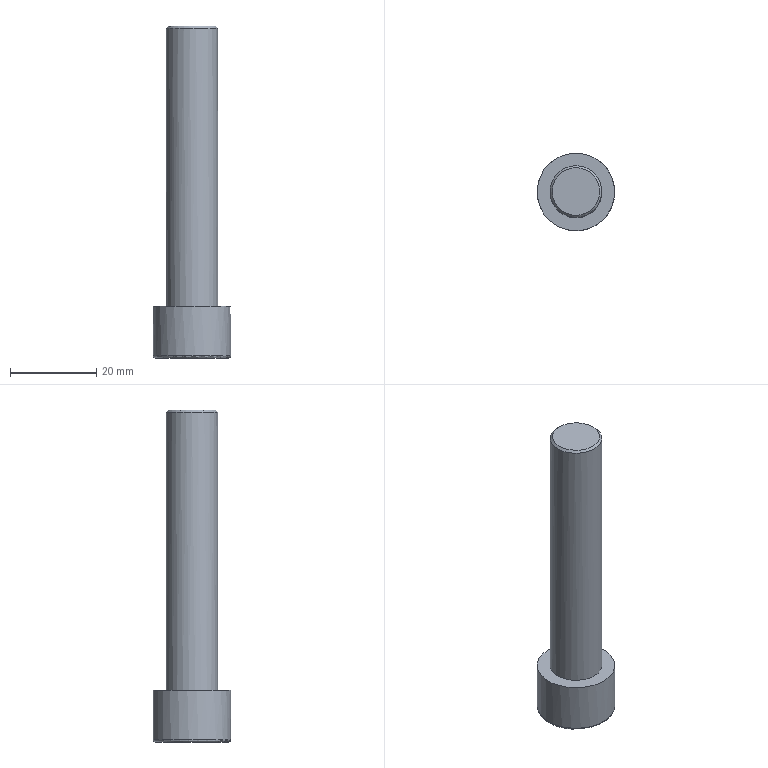Part | NX | features 模具.stp<1>[68] 2 | 1 solid | 14 faces | box 18 x 18 x 77 mm | volume 9878 mm3 | plane 10 | cylinder 2 | cone 1 | torus 1 | commonest cylinder face diameters 12 x1 18 x1
STEP:
#1=CARTESIAN_POINT('',(-5.,-231.113,-93.5));
#2=VERTEX_POINT('',#1);
#3=CARTESIAN_POINT('',(0.,-228.226,-93.5));
#4=VERTEX_POINT('',#3);
#5=CARTESIAN_POINT('',(0.,-228.226,-93.5));
#6=DIRECTION('',(0.866,0.5,0.));
#7=VECTOR('',#6,1000.);
#8=LINE('',#5,#7);
#9=EDGE_CURVE('',#2,#4,#8,.T.);
#10=ORIENTED_EDGE('',*,*,#9,.T.);
#11=CARTESIAN_POINT('',(5.,-231.113,-93.5));
#12=VERTEX_POINT('',#11);
#13=CARTESIAN_POINT('',(5.,-231.113,-93.5));
#14=DIRECTION('',(0.866,-0.5,0.));
#15=VECTOR('',#14,1000.);
#16=LINE('',#13,#15);
#17=EDGE_CURVE('',#4,#12,#16,.T.);
#18=ORIENTED_EDGE('',*,*,#17,.T.);
#19=CARTESIAN_POINT('',(5.,-236.887,-93.5));
#20=VERTEX_POINT('',#19);
#21=CARTESIAN_POINT('',(5.,-236.887,-93.5));
#22=DIRECTION('',(0.,-1.,0.));
#23=VECTOR('',#22,1000.);
#24=LINE('',#21,#23);
#25=EDGE_CURVE('',#12,#20,#24,.T.);
#26=ORIENTED_EDGE('',*,*,#25,.T.);
#27=CARTESIAN_POINT('',(0.,-239.774,-93.5));
#28=VERTEX_POINT('',#27);
#29=CARTESIAN_POINT('',(0.,-239.774,-93.5));
#30=DIRECTION('',(-0.866,-0.5,0.));
#31=VECTOR('',#30,1000.);
#32=LINE('',#29,#31);
#33=EDGE_CURVE('',#20,#28,#32,.T.);
#34=ORIENTED_EDGE('',*,*,#33,.T.);
#35=CARTESIAN_POINT('',(-5.,-236.887,-93.5));
#36=VERTEX_POINT('',#35);
#37=CARTESIAN_POINT('',(-5.,-236.887,-93.5));
#38=DIRECTION('',(-0.866,0.5,0.));
#39=VECTOR('',#38,1000.);
#40=LINE('',#37,#39);
#41=EDGE_CURVE('',#28,#36,#40,.T.);
#42=ORIENTED_EDGE('',*,*,#41,.T.);
#43=CARTESIAN_POINT('',(-5.,-231.113,-93.5));
#44=DIRECTION('',(0.,1.,0.));
#45=VECTOR('',#44,1000.);
#46=LINE('',#43,#45);
#47=EDGE_CURVE('',#36,#2,#46,.T.);
#48=ORIENTED_EDGE('',*,*,#47,.T.);
#49=EDGE_LOOP('',(#10,#18,#26,#34,#42,#48));
#50=FACE_BOUND('',#49,.T.);
#51=CARTESIAN_POINT('',(0.,-234.,-93.5));
#52=DIRECTION('',(0.,0.,1.));
#53=DIRECTION('',(1.,0.,0.));
#54=AXIS2_PLACEMENT_3D('',#51,#52,#53);
#55=PLANE('',#54);
#56=ADVANCED_FACE('',(#50),#55,.F.);
#57=CARTESIAN_POINT('',(-5.,-231.113,-99.5));
#58=VERTEX_POINT('',#57);
#59=CARTESIAN_POINT('',(0.,-228.226,-99.5));
#60=VERTEX_POINT('',#59);
#61=CARTESIAN_POINT('',(0.,-228.226,-99.5));
#62=DIRECTION('',(0.866,0.5,0.));
#63=VECTOR('',#62,1000.);
#64=LINE('',#61,#63);
#65=EDGE_CURVE('',#58,#60,#64,.T.);
#66=ORIENTED_EDGE('',*,*,#65,.T.);
#67=CARTESIAN_POINT('',(0.,-228.226,-93.5));
#68=DIRECTION('',(0.,0.,1.));
#69=VECTOR('',#68,1000.);
#70=LINE('',#67,#69);
#71=EDGE_CURVE('',#60,#4,#70,.T.);
#72=ORIENTED_EDGE('',*,*,#71,.T.);
#73=ORIENTED_EDGE('',*,*,#9,.F.);
#74=CARTESIAN_POINT('',(-5.,-231.113,-93.5));
#75=DIRECTION('',(0.,0.,1.));
#76=VECTOR('',#75,1000.);
#77=LINE('',#74,#76);
#78=EDGE_CURVE('',#58,#2,#77,.T.);
#79=ORIENTED_EDGE('',*,*,#78,.F.);
#80=EDGE_LOOP('',(#66,#72,#73,#79));
#81=FACE_BOUND('',#80,.T.);
#82=CARTESIAN_POINT('',(-2.5,-229.67,-96.5));
#83=DIRECTION('',(-0.5,0.866,0.));
#84=DIRECTION('',(0.,0.,1.));
#85=AXIS2_PLACEMENT_3D('',#82,#83,#84);
#86=PLANE('',#85);
#87=ADVANCED_FACE('',(#81),#86,.F.);
#88=CARTESIAN_POINT('',(-5.,-236.887,-99.5));
#89=VERTEX_POINT('',#88);
#90=CARTESIAN_POINT('',(-5.,-231.113,-99.5));
#91=DIRECTION('',(0.,1.,0.));
#92=VECTOR('',#91,1000.);
#93=LINE('',#90,#92);
#94=EDGE_CURVE('',#89,#58,#93,.T.);
#95=ORIENTED_EDGE('',*,*,#94,.T.);
#96=ORIENTED_EDGE('',*,*,#78,.T.);
#97=ORIENTED_EDGE('',*,*,#47,.F.);
#98=CARTESIAN_POINT('',(-5.,-236.887,-93.5));
#99=DIRECTION('',(0.,0.,1.));
#100=VECTOR('',#99,1000.);
#101=LINE('',#98,#100);
#102=EDGE_CURVE('',#89,#36,#101,.T.);
#103=ORIENTED_EDGE('',*,*,#102,.F.);
#104=EDGE_LOOP('',(#95,#96,#97,#103));
#105=FACE_BOUND('',#104,.T.);
#106=CARTESIAN_POINT('',(-5.,-234.,-96.5));
#107=DIRECTION('',(-1.,0.,0.));
#108=DIRECTION('',(0.,0.,1.));
#109=AXIS2_PLACEMENT_3D('',#106,#107,#108);
#110=PLANE('',#109);
#111=ADVANCED_FACE('',(#105),#110,.F.);
#112=CARTESIAN_POINT('',(0.,-239.774,-99.5));
#113=VERTEX_POINT('',#112);
#114=CARTESIAN_POINT('',(-5.,-236.887,-99.5));
#115=DIRECTION('',(-0.866,0.5,0.));
#116=VECTOR('',#115,1000.);
#117=LINE('',#114,#116);
#118=EDGE_CURVE('',#113,#89,#117,.T.);
#119=ORIENTED_EDGE('',*,*,#118,.T.);
#120=ORIENTED_EDGE('',*,*,#102,.T.);
#121=ORIENTED_EDGE('',*,*,#41,.F.);
#122=CARTESIAN_POINT('',(0.,-239.774,-93.5));
#123=DIRECTION('',(0.,0.,1.));
#124=VECTOR('',#123,1000.);
#125=LINE('',#122,#124);
#126=EDGE_CURVE('',#113,#28,#125,.T.);
#127=ORIENTED_EDGE('',*,*,#126,.F.);
#128=EDGE_LOOP('',(#119,#120,#121,#127));
#129=FACE_BOUND('',#128,.T.);
#130=CARTESIAN_POINT('',(-2.5,-238.33,-96.5));
#131=DIRECTION('',(-0.5,-0.866,0.));
#132=DIRECTION('',(-0.866,0.5,0.));
#133=AXIS2_PLACEMENT_3D('',#130,#131,#132);
#134=PLANE('',#133);
#135=ADVANCED_FACE('',(#129),#134,.F.);
#136=CARTESIAN_POINT('',(5.,-236.887,-99.5));
#137=VERTEX_POINT('',#136);
#138=CARTESIAN_POINT('',(0.,-239.774,-99.5));
#139=DIRECTION('',(-0.866,-0.5,0.));
#140=VECTOR('',#139,1000.);
#141=LINE('',#138,#140);
#142=EDGE_CURVE('',#137,#113,#141,.T.);
#143=ORIENTED_EDGE('',*,*,#142,.T.);
#144=ORIENTED_EDGE('',*,*,#126,.T.);
#145=ORIENTED_EDGE('',*,*,#33,.F.);
#146=CARTESIAN_POINT('',(5.,-236.887,-93.5));
#147=DIRECTION('',(0.,0.,1.));
#148=VECTOR('',#147,1000.);
#149=LINE('',#146,#148);
#150=EDGE_CURVE('',#137,#20,#149,.T.);
#151=ORIENTED_EDGE('',*,*,#150,.F.);
#152=EDGE_LOOP('',(#143,#144,#145,#151));
#153=FACE_BOUND('',#152,.T.);
#154=CARTESIAN_POINT('',(2.5,-238.33,-96.5));
#155=DIRECTION('',(0.5,-0.866,0.));
#156=DIRECTION('',(0.,0.,-1.));
#157=AXIS2_PLACEMENT_3D('',#154,#155,#156);
#158=PLANE('',#157);
#159=ADVANCED_FACE('',(#153),#158,.F.);
#160=CARTESIAN_POINT('',(5.,-231.113,-99.5));
#161=VERTEX_POINT('',#160);
#162=CARTESIAN_POINT('',(5.,-236.887,-99.5));
#163=DIRECTION('',(0.,-1.,0.));
#164=VECTOR('',#163,1000.);
#165=LINE('',#162,#164);
#166=EDGE_CURVE('',#161,#137,#165,.T.);
#167=ORIENTED_EDGE('',*,*,#166,.T.);
#168=ORIENTED_EDGE('',*,*,#150,.T.);
#169=ORIENTED_EDGE('',*,*,#25,.F.);
#170=CARTESIAN_POINT('',(5.,-231.113,-93.5));
#171=DIRECTION('',(0.,0.,1.));
#172=VECTOR('',#171,1000.);
#173=LINE('',#170,#172);
#174=EDGE_CURVE('',#161,#12,#173,.T.);
#175=ORIENTED_EDGE('',*,*,#174,.F.);
#176=EDGE_LOOP('',(#167,#168,#169,#175));
#177=FACE_BOUND('',#176,.T.);
#178=CARTESIAN_POINT('',(5.,-234.,-96.5));
#179=DIRECTION('',(1.,0.,0.));
#180=DIRECTION('',(0.,0.,-1.));
#181=AXIS2_PLACEMENT_3D('',#178,#179,#180);
#182=PLANE('',#181);
#183=ADVANCED_FACE('',(#177),#182,.F.);
#184=CARTESIAN_POINT('',(5.,-231.113,-99.5));
#185=DIRECTION('',(0.866,-0.5,0.));
#186=VECTOR('',#185,1000.);
#187=LINE('',#184,#186);
#188=EDGE_CURVE('',#60,#161,#187,.T.);
#189=ORIENTED_EDGE('',*,*,#188,.T.);
#190=ORIENTED_EDGE('',*,*,#174,.T.);
#191=ORIENTED_EDGE('',*,*,#17,.F.);
#192=ORIENTED_EDGE('',*,*,#71,.F.);
#193=EDGE_LOOP('',(#189,#190,#191,#192));
#194=FACE_BOUND('',#193,.T.);
#195=CARTESIAN_POINT('',(2.5,-229.67,-96.5));
#196=DIRECTION('',(0.5,0.866,0.));
#197=DIRECTION('',(0.,0.,-1.));
#198=AXIS2_PLACEMENT_3D('',#195,#196,#197);
#199=PLANE('',#198);
#200=ADVANCED_FACE('',(#194),#199,.F.);
#201=CARTESIAN_POINT('',(-6.,-234.,-23.));
#202=VERTEX_POINT('',#201);
#203=CARTESIAN_POINT('',(0.,-234.,-23.));
#204=DIRECTION('',(0.,0.,-1.));
#205=DIRECTION('',(-1.,0.,0.));
#206=AXIS2_PLACEMENT_3D('',#203,#204,#205);
#207=CIRCLE('',#206,6.);
#208=EDGE_CURVE('',#202,#202,#207,.T.);
#209=ORIENTED_EDGE('',*,*,#208,.F.);
#210=EDGE_LOOP('',(#209));
#211=FACE_BOUND('',#210,.T.);
#212=CARTESIAN_POINT('',(-5.5,-234.,-22.5));
#213=VERTEX_POINT('',#212);
#214=CARTESIAN_POINT('',(0.,-234.,-22.5));
#215=DIRECTION('',(0.,0.,1.));
#216=DIRECTION('',(-1.,0.,0.));
#217=AXIS2_PLACEMENT_3D('',#214,#215,#216);
#218=CIRCLE('',#217,5.5);
#219=EDGE_CURVE('',#213,#213,#218,.T.);
#220=ORIENTED_EDGE('',*,*,#219,.F.);
#221=EDGE_LOOP('',(#220));
#222=FACE_BOUND('',#221,.T.);
#223=CARTESIAN_POINT('',(0.,-234.,-23.));
#224=DIRECTION('',(0.,0.,-1.));
#225=DIRECTION('',(1.,0.,0.));
#226=AXIS2_PLACEMENT_3D('',#223,#224,#225);
#227=CONICAL_SURFACE('',#226,6.,0.7854);
#228=ADVANCED_FACE('',(#211,#222),#227,.T.);
#229=CARTESIAN_POINT('',(0.,-228.,-87.5));
#230=VERTEX_POINT('',#229);
#231=CARTESIAN_POINT('',(0.,-234.,-87.5));
#232=DIRECTION('',(0.,0.,1.));
#233=DIRECTION('',(0.,1.,0.));
#234=AXIS2_PLACEMENT_3D('',#231,#232,#233);
#235=CIRCLE('',#234,6.);
#236=EDGE_CURVE('',#230,#230,#235,.T.);
#237=ORIENTED_EDGE('',*,*,#236,.T.);
#238=EDGE_LOOP('',(#237));
#239=FACE_BOUND('',#238,.T.);
#240=ORIENTED_EDGE('',*,*,#208,.T.);
#241=EDGE_LOOP('',(#240));
#242=FACE_BOUND('',#241,.T.);
#243=CARTESIAN_POINT('',(0.,-234.,-47.5));
#244=DIRECTION('',(0.,0.,-1.));
#245=DIRECTION('',(0.,1.,0.));
#246=AXIS2_PLACEMENT_3D('',#243,#244,#245);
#247=CYLINDRICAL_SURFACE('',#246,6.);
#248=ADVANCED_FACE('',(#239,#242),#247,.T.);
#249=ORIENTED_EDGE('',*,*,#219,.T.);
#250=EDGE_LOOP('',(#249));
#251=FACE_BOUND('',#250,.T.);
#252=CARTESIAN_POINT('',(0.,-234.,-22.5));
#253=DIRECTION('',(0.,0.,1.));
#254=DIRECTION('',(1.,0.,0.));
#255=AXIS2_PLACEMENT_3D('',#252,#253,#254);
#256=PLANE('',#255);
#257=ADVANCED_FACE('',(#251),#256,.T.);
#258=CARTESIAN_POINT('',(9.,-234.,-99.));
#259=VERTEX_POINT('',#258);
#260=CARTESIAN_POINT('',(0.,-234.,-99.));
#261=DIRECTION('',(0.,0.,1.));
#262=DIRECTION('',(1.,0.,0.));
#263=AXIS2_PLACEMENT_3D('',#260,#261,#262);
#264=CIRCLE('',#263,9.);
#265=EDGE_CURVE('',#259,#259,#264,.T.);
#266=ORIENTED_EDGE('',*,*,#265,.F.);
#267=EDGE_LOOP('',(#266));
#268=FACE_BOUND('',#267,.T.);
#269=CARTESIAN_POINT('',(8.5,-234.,-99.5));
#270=VERTEX_POINT('',#269);
#271=CARTESIAN_POINT('',(0.,-234.,-99.5));
#272=DIRECTION('',(0.,0.,-1.));
#273=DIRECTION('',(1.,0.,0.));
#274=AXIS2_PLACEMENT_3D('',#271,#272,#273);
#275=CIRCLE('',#274,8.5);
#276=EDGE_CURVE('',#270,#270,#275,.T.);
#277=ORIENTED_EDGE('',*,*,#276,.F.);
#278=EDGE_LOOP('',(#277));
#279=FACE_BOUND('',#278,.T.);
#280=CARTESIAN_POINT('',(0.,-234.,-99.));
#281=DIRECTION('',(0.,0.,-1.));
#282=DIRECTION('',(1.,0.,0.));
#283=AXIS2_PLACEMENT_3D('',#280,#281,#282);
#284=TOROIDAL_SURFACE('',#283,8.5,0.5);
#285=ADVANCED_FACE('',(#268,#279),#284,.T.);
#286=CARTESIAN_POINT('',(0.,-225.,-87.5));
#287=VERTEX_POINT('',#286);
#288=CARTESIAN_POINT('',(0.,-234.,-87.5));
#289=DIRECTION('',(0.,0.,-1.));
#290=DIRECTION('',(0.,1.,0.));
#291=AXIS2_PLACEMENT_3D('',#288,#289,#290);
#292=CIRCLE('',#291,9.);
#293=EDGE_CURVE('',#287,#287,#292,.T.);
#294=ORIENTED_EDGE('',*,*,#293,.T.);
#295=EDGE_LOOP('',(#294));
#296=FACE_BOUND('',#295,.T.);
#297=ORIENTED_EDGE('',*,*,#265,.T.);
#298=EDGE_LOOP('',(#297));
#299=FACE_BOUND('',#298,.T.);
#300=CARTESIAN_POINT('',(0.,-234.,-87.5));
#301=DIRECTION('',(0.,0.,-1.));
#302=DIRECTION('',(0.,1.,0.));
#303=AXIS2_PLACEMENT_3D('',#300,#301,#302);
#304=CYLINDRICAL_SURFACE('',#303,9.);
#305=ADVANCED_FACE('',(#296,#299),#304,.T.);
#306=ORIENTED_EDGE('',*,*,#293,.F.);
#307=EDGE_LOOP('',(#306));
#308=FACE_BOUND('',#307,.T.);
#309=ORIENTED_EDGE('',*,*,#236,.F.);
#310=EDGE_LOOP('',(#309));
#311=FACE_BOUND('',#310,.T.);
#312=CARTESIAN_POINT('',(0.,-234.,-87.5));
#313=DIRECTION('',(0.,0.,1.));
#314=DIRECTION('',(1.,0.,0.));
#315=AXIS2_PLACEMENT_3D('',#312,#313,#314);
#316=PLANE('',#315);
#317=ADVANCED_FACE('',(#308,#311),#316,.T.);
#318=ORIENTED_EDGE('',*,*,#276,.T.);
#319=EDGE_LOOP('',(#318));
#320=FACE_BOUND('',#319,.T.);
#321=ORIENTED_EDGE('',*,*,#188,.F.);
#322=ORIENTED_EDGE('',*,*,#65,.F.);
#323=ORIENTED_EDGE('',*,*,#94,.F.);
#324=ORIENTED_EDGE('',*,*,#118,.F.);
#325=ORIENTED_EDGE('',*,*,#142,.F.);
#326=ORIENTED_EDGE('',*,*,#166,.F.);
#327=EDGE_LOOP('',(#321,#322,#323,#324,#325,#326));
#328=FACE_BOUND('',#327,.T.);
#329=CARTESIAN_POINT('',(0.,-234.,-99.5));
#330=DIRECTION('',(0.,0.,-1.));
#331=DIRECTION('',(0.,-1.,0.));
#332=AXIS2_PLACEMENT_3D('',#329,#330,#331);
#333=PLANE('',#332);
#334=ADVANCED_FACE('',(#320,#328),#333,.T.);
#335=CLOSED_SHELL('',(#56,#87,#111,#135,#159,#183,#200,#228,#248,#257,#285,#305,#317,#334));
#336=MANIFOLD_SOLID_BREP('',#335);
#337=(LENGTH_UNIT()NAMED_UNIT(*)SI_UNIT(.MILLI.,.METRE.));
#338=UNCERTAINTY_MEASURE_WITH_UNIT(LENGTH_MEASURE(0.00001),#337,'','');
#339=(NAMED_UNIT(*)PLANE_ANGLE_UNIT()SI_UNIT($,.RADIAN.));
#340=(NAMED_UNIT(*)SI_UNIT($,.STERADIAN.)SOLID_ANGLE_UNIT());
#341=(GEOMETRIC_REPRESENTATION_CONTEXT(3)GLOBAL_UNCERTAINTY_ASSIGNED_CONTEXT((#338))GLOBAL_UNIT_ASSIGNED_CONTEXT((#337,#339,#340))REPRESENTATION_CONTEXT('',''));
#342=ADVANCED_BREP_SHAPE_REPRESENTATION('',(#336),#341);